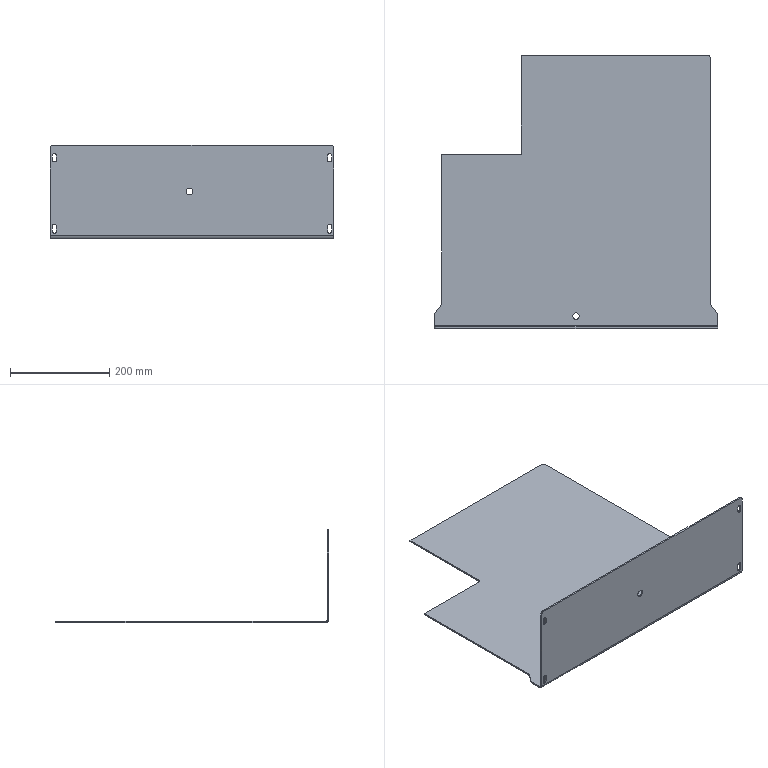Part | SolidWorks | features Fillet 3, ICE 2, FlatPattern 1, SMBaseFlange 1, SheetMetal 1 | 1 solid | 52 faces | box 570 x 550 x 188 mm | volume 1109133 mm3 | cylinder 26 | plane 26 | commonest cylinder face diameters 8.5 x12 20 x4 10 x3 6 x2 13.2 x2 14 x2